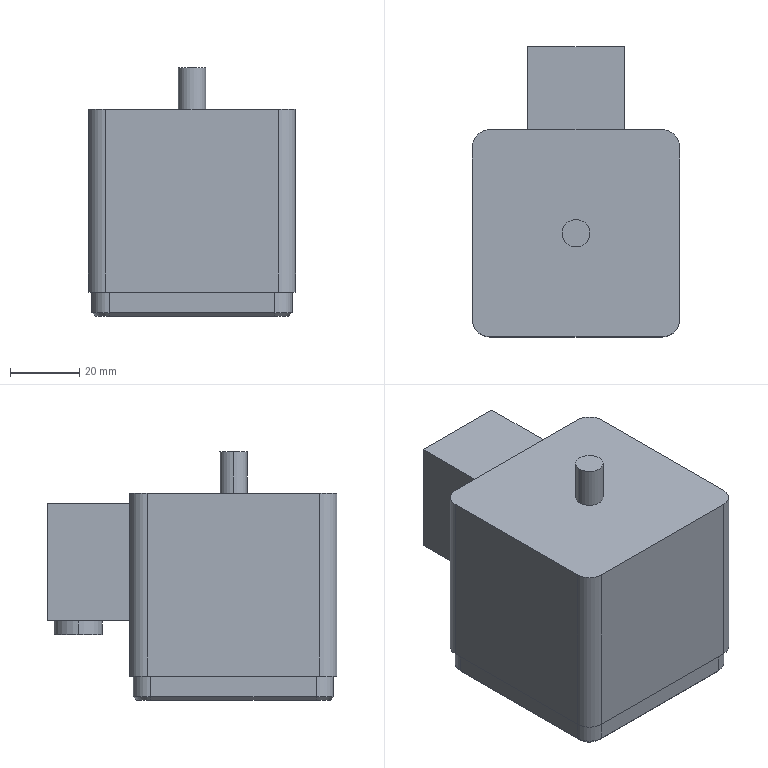Part | SolidWorks | features ICE 4, Fillet 2, Chamfer 1, Extrusion 1 | 1 solid | 38 faces | box 60 x 84 x 72 mm | volume 237017 mm3 | plane 22 | cylinder 12 | cone 4 | commonest cylinder face diameters 10 x8 8 x2 14 x2
STEP:
#1=CARTESIAN_POINT('',(-7.,44.945,23.));
#2=VERTEX_POINT('',#1);
#3=CARTESIAN_POINT('',(7.,44.945,23.));
#4=VERTEX_POINT('',#3);
#5=CARTESIAN_POINT('',(0.,44.945,23.));
#6=DIRECTION('',(0.,0.,-1.));
#7=DIRECTION('',(-1.,0.,0.));
#8=AXIS2_PLACEMENT_3D('',#5,#6,#7);
#9=CIRCLE('',#8,7.);
#10=EDGE_CURVE('',#2,#4,#9,.T.);
#11=ORIENTED_EDGE('',*,*,#10,.T.);
#12=CARTESIAN_POINT('',(7.,44.945,19.));
#13=VERTEX_POINT('',#12);
#14=CARTESIAN_POINT('',(7.,44.945,23.));
#15=DIRECTION('',(0.,0.,-1.));
#16=VECTOR('',#15,1000.);
#17=LINE('',#14,#16);
#18=EDGE_CURVE('',#4,#13,#17,.T.);
#19=ORIENTED_EDGE('',*,*,#18,.T.);
#20=CARTESIAN_POINT('',(-7.,44.945,19.));
#21=VERTEX_POINT('',#20);
#22=CARTESIAN_POINT('',(0.,44.945,19.));
#23=DIRECTION('',(0.,0.,-1.));
#24=DIRECTION('',(-1.,0.,0.));
#25=AXIS2_PLACEMENT_3D('',#22,#23,#24);
#26=CIRCLE('',#25,7.);
#27=EDGE_CURVE('',#21,#13,#26,.T.);
#28=ORIENTED_EDGE('',*,*,#27,.F.);
#29=CARTESIAN_POINT('',(-7.,44.945,23.));
#30=DIRECTION('',(0.,0.,-1.));
#31=VECTOR('',#30,1000.);
#32=LINE('',#29,#31);
#33=EDGE_CURVE('',#2,#21,#32,.T.);
#34=ORIENTED_EDGE('',*,*,#33,.F.);
#35=EDGE_LOOP('',(#11,#19,#28,#34));
#36=FACE_OUTER_BOUND('',#35,.T.);
#37=CARTESIAN_POINT('',(0.,44.945,23.));
#38=DIRECTION('',(0.,0.,-1.));
#39=DIRECTION('',(-1.,0.,0.));
#40=AXIS2_PLACEMENT_3D('',#37,#38,#39);
#41=CYLINDRICAL_SURFACE('',#40,7.);
#42=ADVANCED_FACE('',(#36),#41,.T.);
#43=CARTESIAN_POINT('',(4.,0.,72.));
#44=VERTEX_POINT('',#43);
#45=CARTESIAN_POINT('',(-4.,0.,72.));
#46=VERTEX_POINT('',#45);
#47=CARTESIAN_POINT('',(0.,0.,72.));
#48=DIRECTION('',(0.,0.,1.));
#49=DIRECTION('',(1.,0.,0.));
#50=AXIS2_PLACEMENT_3D('',#47,#48,#49);
#51=CIRCLE('',#50,4.);
#52=EDGE_CURVE('',#44,#46,#51,.T.);
#53=ORIENTED_EDGE('',*,*,#52,.F.);
#54=CARTESIAN_POINT('',(4.,0.,60.));
#55=VERTEX_POINT('',#54);
#56=CARTESIAN_POINT('',(4.,0.,72.));
#57=DIRECTION('',(0.,0.,-1.));
#58=VECTOR('',#57,1000.);
#59=LINE('',#56,#58);
#60=EDGE_CURVE('',#44,#55,#59,.T.);
#61=ORIENTED_EDGE('',*,*,#60,.T.);
#62=CARTESIAN_POINT('',(-4.,0.,60.));
#63=VERTEX_POINT('',#62);
#64=CARTESIAN_POINT('',(0.,0.,60.));
#65=DIRECTION('',(0.,0.,1.));
#66=DIRECTION('',(1.,0.,0.));
#67=AXIS2_PLACEMENT_3D('',#64,#65,#66);
#68=CIRCLE('',#67,4.);
#69=EDGE_CURVE('',#55,#63,#68,.T.);
#70=ORIENTED_EDGE('',*,*,#69,.T.);
#71=CARTESIAN_POINT('',(-4.,0.,72.));
#72=DIRECTION('',(0.,0.,-1.));
#73=VECTOR('',#72,1000.);
#74=LINE('',#71,#73);
#75=EDGE_CURVE('',#46,#63,#74,.T.);
#76=ORIENTED_EDGE('',*,*,#75,.F.);
#77=EDGE_LOOP('',(#53,#61,#70,#76));
#78=FACE_OUTER_BOUND('',#77,.T.);
#79=CARTESIAN_POINT('',(0.,0.,72.));
#80=DIRECTION('',(0.,0.,-1.));
#81=DIRECTION('',(-1.,0.,0.));
#82=AXIS2_PLACEMENT_3D('',#79,#80,#81);
#83=CYLINDRICAL_SURFACE('',#82,4.);
#84=ADVANCED_FACE('',(#78),#83,.T.);
#85=CARTESIAN_POINT('',(14.,54.,23.));
#86=VERTEX_POINT('',#85);
#87=CARTESIAN_POINT('',(14.,30.,23.));
#88=VERTEX_POINT('',#87);
#89=CARTESIAN_POINT('',(14.,54.,23.));
#90=DIRECTION('',(0.,-1.,0.));
#91=VECTOR('',#90,1000.);
#92=LINE('',#89,#91);
#93=EDGE_CURVE('',#86,#88,#92,.T.);
#94=ORIENTED_EDGE('',*,*,#93,.F.);
#95=CARTESIAN_POINT('',(14.,54.,57.));
#96=VERTEX_POINT('',#95);
#97=CARTESIAN_POINT('',(14.,54.,57.));
#98=DIRECTION('',(0.,0.,-1.));
#99=VECTOR('',#98,1000.);
#100=LINE('',#97,#99);
#101=EDGE_CURVE('',#96,#86,#100,.T.);
#102=ORIENTED_EDGE('',*,*,#101,.F.);
#103=CARTESIAN_POINT('',(14.,30.,57.));
#104=VERTEX_POINT('',#103);
#105=CARTESIAN_POINT('',(14.,54.,57.));
#106=DIRECTION('',(0.,-1.,0.));
#107=VECTOR('',#106,1000.);
#108=LINE('',#105,#107);
#109=EDGE_CURVE('',#96,#104,#108,.T.);
#110=ORIENTED_EDGE('',*,*,#109,.T.);
#111=CARTESIAN_POINT('',(14.,30.,57.));
#112=DIRECTION('',(0.,0.,-1.));
#113=VECTOR('',#112,1000.);
#114=LINE('',#111,#113);
#115=EDGE_CURVE('',#104,#88,#114,.T.);
#116=ORIENTED_EDGE('',*,*,#115,.T.);
#117=EDGE_LOOP('',(#94,#102,#110,#116));
#118=FACE_OUTER_BOUND('',#117,.T.);
#119=CARTESIAN_POINT('',(14.,54.,57.));
#120=DIRECTION('',(-1.,0.,0.));
#121=DIRECTION('',(0.,0.,1.));
#122=AXIS2_PLACEMENT_3D('',#119,#120,#121);
#123=PLANE('',#122);
#124=ADVANCED_FACE('',(#118),#123,.F.);
#125=CARTESIAN_POINT('',(-14.,30.,23.));
#126=VERTEX_POINT('',#125);
#127=CARTESIAN_POINT('',(-14.,54.,23.));
#128=VERTEX_POINT('',#127);
#129=CARTESIAN_POINT('',(-14.,54.,23.));
#130=DIRECTION('',(0.,1.,0.));
#131=VECTOR('',#130,1000.);
#132=LINE('',#129,#131);
#133=EDGE_CURVE('',#126,#128,#132,.T.);
#134=ORIENTED_EDGE('',*,*,#133,.F.);
#135=CARTESIAN_POINT('',(-14.,30.,57.));
#136=VERTEX_POINT('',#135);
#137=CARTESIAN_POINT('',(-14.,30.,57.));
#138=DIRECTION('',(0.,0.,1.));
#139=VECTOR('',#138,1000.);
#140=LINE('',#137,#139);
#141=EDGE_CURVE('',#126,#136,#140,.T.);
#142=ORIENTED_EDGE('',*,*,#141,.T.);
#143=CARTESIAN_POINT('',(-14.,54.,57.));
#144=VERTEX_POINT('',#143);
#145=CARTESIAN_POINT('',(-14.,54.,57.));
#146=DIRECTION('',(0.,-1.,0.));
#147=VECTOR('',#146,1000.);
#148=LINE('',#145,#147);
#149=EDGE_CURVE('',#144,#136,#148,.T.);
#150=ORIENTED_EDGE('',*,*,#149,.F.);
#151=CARTESIAN_POINT('',(-14.,54.,57.));
#152=DIRECTION('',(0.,0.,1.));
#153=VECTOR('',#152,1000.);
#154=LINE('',#151,#153);
#155=EDGE_CURVE('',#128,#144,#154,.T.);
#156=ORIENTED_EDGE('',*,*,#155,.F.);
#157=EDGE_LOOP('',(#134,#142,#150,#156));
#158=FACE_OUTER_BOUND('',#157,.T.);
#159=CARTESIAN_POINT('',(-14.,54.,57.));
#160=DIRECTION('',(1.,0.,0.));
#161=DIRECTION('',(0.,0.,-1.));
#162=AXIS2_PLACEMENT_3D('',#159,#160,#161);
#163=PLANE('',#162);
#164=ADVANCED_FACE('',(#158),#163,.F.);
#165=CARTESIAN_POINT('',(0.,54.,23.));
#166=DIRECTION('',(1.,0.,0.));
#167=VECTOR('',#166,1000.);
#168=LINE('',#165,#167);
#169=EDGE_CURVE('',#128,#86,#168,.T.);
#170=ORIENTED_EDGE('',*,*,#169,.F.);
#171=ORIENTED_EDGE('',*,*,#155,.T.);
#172=CARTESIAN_POINT('',(14.,54.,57.));
#173=DIRECTION('',(1.,0.,0.));
#174=VECTOR('',#173,1000.);
#175=LINE('',#172,#174);
#176=EDGE_CURVE('',#144,#96,#175,.T.);
#177=ORIENTED_EDGE('',*,*,#176,.T.);
#178=ORIENTED_EDGE('',*,*,#101,.T.);
#179=EDGE_LOOP('',(#170,#171,#177,#178));
#180=FACE_OUTER_BOUND('',#179,.T.);
#181=CARTESIAN_POINT('',(0.,54.,0.));
#182=DIRECTION('',(0.,-1.,0.));
#183=DIRECTION('',(0.,0.,-1.));
#184=AXIS2_PLACEMENT_3D('',#181,#182,#183);
#185=PLANE('',#184);
#186=ADVANCED_FACE('',(#180),#185,.F.);
#187=ORIENTED_EDGE('',*,*,#141,.F.);
#188=CARTESIAN_POINT('',(22.114,30.,23.));
#189=DIRECTION('',(-1.,0.,0.));
#190=VECTOR('',#189,1000.);
#191=LINE('',#188,#190);
#192=EDGE_CURVE('',#88,#126,#191,.T.);
#193=ORIENTED_EDGE('',*,*,#192,.F.);
#194=ORIENTED_EDGE('',*,*,#115,.F.);
#195=CARTESIAN_POINT('',(14.,30.,57.));
#196=DIRECTION('',(1.,0.,0.));
#197=VECTOR('',#196,1000.);
#198=LINE('',#195,#197);
#199=EDGE_CURVE('',#136,#104,#198,.T.);
#200=ORIENTED_EDGE('',*,*,#199,.F.);
#201=EDGE_LOOP('',(#187,#193,#194,#200));
#202=FACE_BOUND('',#201,.T.);
#203=CARTESIAN_POINT('',(-25.,30.,7.));
#204=VERTEX_POINT('',#203);
#205=CARTESIAN_POINT('',(25.,30.,7.));
#206=VERTEX_POINT('',#205);
#207=CARTESIAN_POINT('',(30.,30.,7.));
#208=DIRECTION('',(1.,0.,0.));
#209=VECTOR('',#208,1000.);
#210=LINE('',#207,#209);
#211=EDGE_CURVE('',#204,#206,#210,.T.);
#212=ORIENTED_EDGE('',*,*,#211,.F.);
#213=CARTESIAN_POINT('',(-25.,30.,60.));
#214=VERTEX_POINT('',#213);
#215=CARTESIAN_POINT('',(-25.,30.,60.));
#216=DIRECTION('',(0.,0.,1.));
#217=VECTOR('',#216,1000.);
#218=LINE('',#215,#217);
#219=EDGE_CURVE('',#204,#214,#218,.T.);
#220=ORIENTED_EDGE('',*,*,#219,.T.);
#221=CARTESIAN_POINT('',(25.,30.,60.));
#222=VERTEX_POINT('',#221);
#223=CARTESIAN_POINT('',(-30.,30.,60.));
#224=DIRECTION('',(-1.,0.,0.));
#225=VECTOR('',#224,1000.);
#226=LINE('',#223,#225);
#227=EDGE_CURVE('',#222,#214,#226,.T.);
#228=ORIENTED_EDGE('',*,*,#227,.F.);
#229=CARTESIAN_POINT('',(25.,30.,60.));
#230=DIRECTION('',(0.,0.,-1.));
#231=VECTOR('',#230,1000.);
#232=LINE('',#229,#231);
#233=EDGE_CURVE('',#222,#206,#232,.T.);
#234=ORIENTED_EDGE('',*,*,#233,.T.);
#235=EDGE_LOOP('',(#212,#220,#228,#234));
#236=FACE_OUTER_BOUND('',#235,.T.);
#237=CARTESIAN_POINT('',(-30.,30.,60.));
#238=DIRECTION('',(0.,-1.,0.));
#239=DIRECTION('',(0.,0.,-1.));
#240=AXIS2_PLACEMENT_3D('',#237,#238,#239);
#241=PLANE('',#240);
#242=ADVANCED_FACE('',(#202,#236),#241,.F.);
#243=CARTESIAN_POINT('',(30.,-25.,60.));
#244=VERTEX_POINT('',#243);
#245=CARTESIAN_POINT('',(30.,25.,60.));
#246=VERTEX_POINT('',#245);
#247=CARTESIAN_POINT('',(30.,30.,60.));
#248=DIRECTION('',(0.,1.,0.));
#249=VECTOR('',#248,1000.);
#250=LINE('',#247,#249);
#251=EDGE_CURVE('',#244,#246,#250,.T.);
#252=ORIENTED_EDGE('',*,*,#251,.F.);
#253=CARTESIAN_POINT('',(30.,-25.,7.));
#254=VERTEX_POINT('',#253);
#255=CARTESIAN_POINT('',(30.,-25.,60.));
#256=DIRECTION('',(0.,0.,-1.));
#257=VECTOR('',#256,1000.);
#258=LINE('',#255,#257);
#259=EDGE_CURVE('',#244,#254,#258,.T.);
#260=ORIENTED_EDGE('',*,*,#259,.T.);
#261=CARTESIAN_POINT('',(30.,25.,7.));
#262=VERTEX_POINT('',#261);
#263=CARTESIAN_POINT('',(30.,30.,7.));
#264=DIRECTION('',(0.,-1.,0.));
#265=VECTOR('',#264,1000.);
#266=LINE('',#263,#265);
#267=EDGE_CURVE('',#262,#254,#266,.T.);
#268=ORIENTED_EDGE('',*,*,#267,.F.);
#269=CARTESIAN_POINT('',(30.,25.,60.));
#270=DIRECTION('',(0.,0.,1.));
#271=VECTOR('',#270,1000.);
#272=LINE('',#269,#271);
#273=EDGE_CURVE('',#262,#246,#272,.T.);
#274=ORIENTED_EDGE('',*,*,#273,.T.);
#275=EDGE_LOOP('',(#252,#260,#268,#274));
#276=FACE_OUTER_BOUND('',#275,.T.);
#277=CARTESIAN_POINT('',(30.,30.,60.));
#278=DIRECTION('',(-1.,0.,0.));
#279=DIRECTION('',(0.,-1.,0.));
#280=AXIS2_PLACEMENT_3D('',#277,#278,#279);
#281=PLANE('',#280);
#282=ADVANCED_FACE('',(#276),#281,.F.);
#283=CARTESIAN_POINT('',(-30.,-25.,7.));
#284=VERTEX_POINT('',#283);
#285=CARTESIAN_POINT('',(-30.,25.,7.));
#286=VERTEX_POINT('',#285);
#287=CARTESIAN_POINT('',(-30.,30.,7.));
#288=DIRECTION('',(0.,1.,0.));
#289=VECTOR('',#288,1000.);
#290=LINE('',#287,#289);
#291=EDGE_CURVE('',#284,#286,#290,.T.);
#292=ORIENTED_EDGE('',*,*,#291,.F.);
#293=CARTESIAN_POINT('',(-30.,-25.,60.));
#294=VERTEX_POINT('',#293);
#295=CARTESIAN_POINT('',(-30.,-25.,60.));
#296=DIRECTION('',(0.,0.,1.));
#297=VECTOR('',#296,1000.);
#298=LINE('',#295,#297);
#299=EDGE_CURVE('',#284,#294,#298,.T.);
#300=ORIENTED_EDGE('',*,*,#299,.T.);
#301=CARTESIAN_POINT('',(-30.,25.,60.));
#302=VERTEX_POINT('',#301);
#303=CARTESIAN_POINT('',(-30.,30.,60.));
#304=DIRECTION('',(0.,-1.,0.));
#305=VECTOR('',#304,1000.);
#306=LINE('',#303,#305);
#307=EDGE_CURVE('',#302,#294,#306,.T.);
#308=ORIENTED_EDGE('',*,*,#307,.F.);
#309=CARTESIAN_POINT('',(-30.,25.,60.));
#310=DIRECTION('',(0.,0.,-1.));
#311=VECTOR('',#310,1000.);
#312=LINE('',#309,#311);
#313=EDGE_CURVE('',#302,#286,#312,.T.);
#314=ORIENTED_EDGE('',*,*,#313,.T.);
#315=EDGE_LOOP('',(#292,#300,#308,#314));
#316=FACE_OUTER_BOUND('',#315,.T.);
#317=CARTESIAN_POINT('',(-30.,30.,60.));
#318=DIRECTION('',(1.,0.,0.));
#319=DIRECTION('',(0.,1.,0.));
#320=AXIS2_PLACEMENT_3D('',#317,#318,#319);
#321=PLANE('',#320);
#322=ADVANCED_FACE('',(#316),#321,.F.);
#323=CARTESIAN_POINT('',(25.,-30.,7.));
#324=VERTEX_POINT('',#323);
#325=CARTESIAN_POINT('',(-25.,-30.,7.));
#326=VERTEX_POINT('',#325);
#327=CARTESIAN_POINT('',(30.,-30.,7.));
#328=DIRECTION('',(-1.,0.,0.));
#329=VECTOR('',#328,1000.);
#330=LINE('',#327,#329);
#331=EDGE_CURVE('',#324,#326,#330,.T.);
#332=ORIENTED_EDGE('',*,*,#331,.F.);
#333=CARTESIAN_POINT('',(25.,-30.,60.));
#334=VERTEX_POINT('',#333);
#335=CARTESIAN_POINT('',(25.,-30.,60.));
#336=DIRECTION('',(0.,0.,1.));
#337=VECTOR('',#336,1000.);
#338=LINE('',#335,#337);
#339=EDGE_CURVE('',#324,#334,#338,.T.);
#340=ORIENTED_EDGE('',*,*,#339,.T.);
#341=CARTESIAN_POINT('',(-25.,-30.,60.));
#342=VERTEX_POINT('',#341);
#343=CARTESIAN_POINT('',(-30.,-30.,60.));
#344=DIRECTION('',(1.,0.,0.));
#345=VECTOR('',#344,1000.);
#346=LINE('',#343,#345);
#347=EDGE_CURVE('',#342,#334,#346,.T.);
#348=ORIENTED_EDGE('',*,*,#347,.F.);
#349=CARTESIAN_POINT('',(-25.,-30.,60.));
#350=DIRECTION('',(0.,0.,-1.));
#351=VECTOR('',#350,1000.);
#352=LINE('',#349,#351);
#353=EDGE_CURVE('',#342,#326,#352,.T.);
#354=ORIENTED_EDGE('',*,*,#353,.T.);
#355=EDGE_LOOP('',(#332,#340,#348,#354));
#356=FACE_OUTER_BOUND('',#355,.T.);
#357=CARTESIAN_POINT('',(-30.,-30.,60.));
#358=DIRECTION('',(0.,1.,0.));
#359=DIRECTION('',(0.,0.,1.));
#360=AXIS2_PLACEMENT_3D('',#357,#358,#359);
#361=PLANE('',#360);
#362=ADVANCED_FACE('',(#356),#361,.F.);
#363=CARTESIAN_POINT('',(0.,0.,60.));
#364=DIRECTION('',(0.,0.,1.));
#365=DIRECTION('',(1.,0.,0.));
#366=AXIS2_PLACEMENT_3D('',#363,#364,#365);
#367=CIRCLE('',#366,4.);
#368=EDGE_CURVE('',#63,#55,#367,.T.);
#369=ORIENTED_EDGE('',*,*,#368,.F.);
#370=ORIENTED_EDGE('',*,*,#69,.F.);
#371=EDGE_LOOP('',(#369,#370));
#372=FACE_BOUND('',#371,.T.);
#373=ORIENTED_EDGE('',*,*,#347,.T.);
#374=CARTESIAN_POINT('',(25.,-25.,60.));
#375=DIRECTION('',(0.,0.,1.));
#376=DIRECTION('',(1.,0.,0.));
#377=AXIS2_PLACEMENT_3D('',#374,#375,#376);
#378=CIRCLE('',#377,5.);
#379=EDGE_CURVE('',#334,#244,#378,.T.);
#380=ORIENTED_EDGE('',*,*,#379,.T.);
#381=ORIENTED_EDGE('',*,*,#251,.T.);
#382=CARTESIAN_POINT('',(25.,25.,60.));
#383=DIRECTION('',(0.,0.,1.));
#384=DIRECTION('',(1.,0.,0.));
#385=AXIS2_PLACEMENT_3D('',#382,#383,#384);
#386=CIRCLE('',#385,5.);
#387=EDGE_CURVE('',#246,#222,#386,.T.);
#388=ORIENTED_EDGE('',*,*,#387,.T.);
#389=ORIENTED_EDGE('',*,*,#227,.T.);
#390=CARTESIAN_POINT('',(-25.,25.,60.));
#391=DIRECTION('',(0.,0.,1.));
#392=DIRECTION('',(1.,0.,0.));
#393=AXIS2_PLACEMENT_3D('',#390,#391,#392);
#394=CIRCLE('',#393,5.);
#395=EDGE_CURVE('',#214,#302,#394,.T.);
#396=ORIENTED_EDGE('',*,*,#395,.T.);
#397=ORIENTED_EDGE('',*,*,#307,.T.);
#398=CARTESIAN_POINT('',(-25.,-25.,60.));
#399=DIRECTION('',(0.,0.,1.));
#400=DIRECTION('',(1.,0.,0.));
#401=AXIS2_PLACEMENT_3D('',#398,#399,#400);
#402=CIRCLE('',#401,5.);
#403=EDGE_CURVE('',#294,#342,#402,.T.);
#404=ORIENTED_EDGE('',*,*,#403,.T.);
#405=EDGE_LOOP('',(#373,#380,#381,#388,#389,#396,#397,#404));
#406=FACE_OUTER_BOUND('',#405,.T.);
#407=CARTESIAN_POINT('',(0.,0.,60.));
#408=DIRECTION('',(0.,0.,1.));
#409=DIRECTION('',(1.,0.,0.));
#410=AXIS2_PLACEMENT_3D('',#407,#408,#409);
#411=PLANE('',#410);
#412=ADVANCED_FACE('',(#372,#406),#411,.T.);
#413=ORIENTED_EDGE('',*,*,#60,.F.);
#414=CARTESIAN_POINT('',(0.,0.,72.));
#415=DIRECTION('',(0.,0.,1.));
#416=DIRECTION('',(1.,0.,0.));
#417=AXIS2_PLACEMENT_3D('',#414,#415,#416);
#418=CIRCLE('',#417,4.);
#419=EDGE_CURVE('',#46,#44,#418,.T.);
#420=ORIENTED_EDGE('',*,*,#419,.F.);
#421=ORIENTED_EDGE('',*,*,#75,.T.);
#422=ORIENTED_EDGE('',*,*,#368,.T.);
#423=EDGE_LOOP('',(#413,#420,#421,#422));
#424=FACE_OUTER_BOUND('',#423,.T.);
#425=CARTESIAN_POINT('',(0.,0.,72.));
#426=DIRECTION('',(0.,0.,-1.));
#427=DIRECTION('',(-1.,0.,0.));
#428=AXIS2_PLACEMENT_3D('',#425,#426,#427);
#429=CYLINDRICAL_SURFACE('',#428,4.);
#430=ADVANCED_FACE('',(#424),#429,.T.);
#431=ORIENTED_EDGE('',*,*,#419,.T.);
#432=ORIENTED_EDGE('',*,*,#52,.T.);
#433=EDGE_LOOP('',(#431,#432));
#434=FACE_OUTER_BOUND('',#433,.T.);
#435=CARTESIAN_POINT('',(0.,0.,72.));
#436=DIRECTION('',(0.,0.,1.));
#437=DIRECTION('',(1.,0.,0.));
#438=AXIS2_PLACEMENT_3D('',#435,#436,#437);
#439=PLANE('',#438);
#440=ADVANCED_FACE('',(#434),#439,.T.);
#441=CARTESIAN_POINT('',(24.,-29.,7.));
#442=VERTEX_POINT('',#441);
#443=CARTESIAN_POINT('',(-24.,-29.,7.));
#444=VERTEX_POINT('',#443);
#445=CARTESIAN_POINT('',(29.,-29.,7.));
#446=DIRECTION('',(-1.,0.,0.));
#447=VECTOR('',#446,1000.);
#448=LINE('',#445,#447);
#449=EDGE_CURVE('',#442,#444,#448,.T.);
#450=ORIENTED_EDGE('',*,*,#449,.F.);
#451=CARTESIAN_POINT('',(29.,-24.,7.));
#452=VERTEX_POINT('',#451);
#453=CARTESIAN_POINT('',(24.,-24.,7.));
#454=DIRECTION('',(0.,0.,1.));
#455=DIRECTION('',(-1.,0.,0.));
#456=AXIS2_PLACEMENT_3D('',#453,#454,#455);
#457=CIRCLE('',#456,5.);
#458=EDGE_CURVE('',#442,#452,#457,.T.);
#459=ORIENTED_EDGE('',*,*,#458,.T.);
#460=CARTESIAN_POINT('',(29.,24.,7.));
#461=VERTEX_POINT('',#460);
#462=CARTESIAN_POINT('',(29.,29.,7.));
#463=DIRECTION('',(0.,-1.,0.));
#464=VECTOR('',#463,1000.);
#465=LINE('',#462,#464);
#466=EDGE_CURVE('',#461,#452,#465,.T.);
#467=ORIENTED_EDGE('',*,*,#466,.F.);
#468=CARTESIAN_POINT('',(24.,29.,7.));
#469=VERTEX_POINT('',#468);
#470=CARTESIAN_POINT('',(24.,24.,7.));
#471=DIRECTION('',(0.,0.,1.));
#472=DIRECTION('',(-1.,0.,0.));
#473=AXIS2_PLACEMENT_3D('',#470,#471,#472);
#474=CIRCLE('',#473,5.);
#475=EDGE_CURVE('',#461,#469,#474,.T.);
#476=ORIENTED_EDGE('',*,*,#475,.T.);
#477=CARTESIAN_POINT('',(-24.,29.,7.));
#478=VERTEX_POINT('',#477);
#479=CARTESIAN_POINT('',(29.,29.,7.));
#480=DIRECTION('',(1.,0.,0.));
#481=VECTOR('',#480,1000.);
#482=LINE('',#479,#481);
#483=EDGE_CURVE('',#478,#469,#482,.T.);
#484=ORIENTED_EDGE('',*,*,#483,.F.);
#485=CARTESIAN_POINT('',(-29.,24.,7.));
#486=VERTEX_POINT('',#485);
#487=CARTESIAN_POINT('',(-24.,24.,7.));
#488=DIRECTION('',(0.,0.,1.));
#489=DIRECTION('',(-1.,0.,0.));
#490=AXIS2_PLACEMENT_3D('',#487,#488,#489);
#491=CIRCLE('',#490,5.);
#492=EDGE_CURVE('',#478,#486,#491,.T.);
#493=ORIENTED_EDGE('',*,*,#492,.T.);
#494=CARTESIAN_POINT('',(-29.,-24.,7.));
#495=VERTEX_POINT('',#494);
#496=CARTESIAN_POINT('',(-29.,29.,7.));
#497=DIRECTION('',(0.,1.,0.));
#498=VECTOR('',#497,1000.);
#499=LINE('',#496,#498);
#500=EDGE_CURVE('',#495,#486,#499,.T.);
#501=ORIENTED_EDGE('',*,*,#500,.F.);
#502=CARTESIAN_POINT('',(-24.,-24.,7.));
#503=DIRECTION('',(0.,0.,1.));
#504=DIRECTION('',(-1.,0.,0.));
#505=AXIS2_PLACEMENT_3D('',#502,#503,#504);
#506=CIRCLE('',#505,5.);
#507=EDGE_CURVE('',#495,#444,#506,.T.);
#508=ORIENTED_EDGE('',*,*,#507,.T.);
#509=EDGE_LOOP('',(#450,#459,#467,#476,#484,#493,#501,#508));
#510=FACE_BOUND('',#509,.T.);
#511=ORIENTED_EDGE('',*,*,#267,.T.);
#512=CARTESIAN_POINT('',(25.,-25.,7.));
#513=DIRECTION('',(0.,0.,-1.));
#514=DIRECTION('',(-1.,0.,0.));
#515=AXIS2_PLACEMENT_3D('',#512,#513,#514);
#516=CIRCLE('',#515,5.);
#517=EDGE_CURVE('',#254,#324,#516,.T.);
#518=ORIENTED_EDGE('',*,*,#517,.T.);
#519=ORIENTED_EDGE('',*,*,#331,.T.);
#520=CARTESIAN_POINT('',(-25.,-25.,7.));
#521=DIRECTION('',(0.,0.,-1.));
#522=DIRECTION('',(-1.,0.,0.));
#523=AXIS2_PLACEMENT_3D('',#520,#521,#522);
#524=CIRCLE('',#523,5.);
#525=EDGE_CURVE('',#326,#284,#524,.T.);
#526=ORIENTED_EDGE('',*,*,#525,.T.);
#527=ORIENTED_EDGE('',*,*,#291,.T.);
#528=CARTESIAN_POINT('',(-25.,25.,7.));
#529=DIRECTION('',(0.,0.,-1.));
#530=DIRECTION('',(-1.,0.,0.));
#531=AXIS2_PLACEMENT_3D('',#528,#529,#530);
#532=CIRCLE('',#531,5.);
#533=EDGE_CURVE('',#286,#204,#532,.T.);
#534=ORIENTED_EDGE('',*,*,#533,.T.);
#535=ORIENTED_EDGE('',*,*,#211,.T.);
#536=CARTESIAN_POINT('',(25.,25.,7.));
#537=DIRECTION('',(0.,0.,-1.));
#538=DIRECTION('',(-1.,0.,0.));
#539=AXIS2_PLACEMENT_3D('',#536,#537,#538);
#540=CIRCLE('',#539,5.);
#541=EDGE_CURVE('',#206,#262,#540,.T.);
#542=ORIENTED_EDGE('',*,*,#541,.T.);
#543=EDGE_LOOP('',(#511,#518,#519,#526,#527,#534,#535,#542));
#544=FACE_OUTER_BOUND('',#543,.T.);
#545=CARTESIAN_POINT('',(0.,0.,7.));
#546=DIRECTION('',(0.,0.,-1.));
#547=DIRECTION('',(-1.,0.,0.));
#548=AXIS2_PLACEMENT_3D('',#545,#546,#547);
#549=PLANE('',#548);
#550=ADVANCED_FACE('',(#510,#544),#549,.T.);
#551=CARTESIAN_POINT('',(-29.,24.,1.));
#552=VERTEX_POINT('',#551);
#553=CARTESIAN_POINT('',(-29.,24.,7.));
#554=DIRECTION('',(0.,0.,-1.));
#555=VECTOR('',#554,1000.);
#556=LINE('',#553,#555);
#557=EDGE_CURVE('',#486,#552,#556,.T.);
#558=ORIENTED_EDGE('',*,*,#557,.T.);
#559=CARTESIAN_POINT('',(-29.,-24.,1.));
#560=VERTEX_POINT('',#559);
#561=CARTESIAN_POINT('',(-29.,-24.,1.));
#562=DIRECTION('',(0.,-1.,0.));
#563=VECTOR('',#562,1000.);
#564=LINE('',#561,#563);
#565=EDGE_CURVE('',#552,#560,#564,.T.);
#566=ORIENTED_EDGE('',*,*,#565,.T.);
#567=CARTESIAN_POINT('',(-29.,-24.,7.));
#568=DIRECTION('',(0.,0.,1.));
#569=VECTOR('',#568,1000.);
#570=LINE('',#567,#569);
#571=EDGE_CURVE('',#560,#495,#570,.T.);
#572=ORIENTED_EDGE('',*,*,#571,.T.);
#573=ORIENTED_EDGE('',*,*,#500,.T.);
#574=EDGE_LOOP('',(#558,#566,#572,#573));
#575=FACE_OUTER_BOUND('',#574,.T.);
#576=CARTESIAN_POINT('',(-29.,29.,7.));
#577=DIRECTION('',(-1.,0.,0.));
#578=DIRECTION('',(0.,-1.,0.));
#579=AXIS2_PLACEMENT_3D('',#576,#577,#578);
#580=PLANE('',#579);
#581=ADVANCED_FACE('',(#575),#580,.T.);
#582=CARTESIAN_POINT('',(-24.,-29.,1.));
#583=VERTEX_POINT('',#582);
#584=CARTESIAN_POINT('',(-24.,-29.,7.));
#585=DIRECTION('',(0.,0.,-1.));
#586=VECTOR('',#585,1000.);
#587=LINE('',#584,#586);
#588=EDGE_CURVE('',#444,#583,#587,.T.);
#589=ORIENTED_EDGE('',*,*,#588,.T.);
#590=CARTESIAN_POINT('',(24.,-29.,1.));
#591=VERTEX_POINT('',#590);
#592=CARTESIAN_POINT('',(24.,-29.,1.));
#593=DIRECTION('',(1.,0.,0.));
#594=VECTOR('',#593,1000.);
#595=LINE('',#592,#594);
#596=EDGE_CURVE('',#583,#591,#595,.T.);
#597=ORIENTED_EDGE('',*,*,#596,.T.);
#598=CARTESIAN_POINT('',(24.,-29.,7.));
#599=DIRECTION('',(0.,0.,1.));
#600=VECTOR('',#599,1000.);
#601=LINE('',#598,#600);
#602=EDGE_CURVE('',#591,#442,#601,.T.);
#603=ORIENTED_EDGE('',*,*,#602,.T.);
#604=ORIENTED_EDGE('',*,*,#449,.T.);
#605=EDGE_LOOP('',(#589,#597,#603,#604));
#606=FACE_OUTER_BOUND('',#605,.T.);
#607=CARTESIAN_POINT('',(29.,-29.,7.));
#608=DIRECTION('',(0.,-1.,0.));
#609=DIRECTION('',(0.,0.,-1.));
#610=AXIS2_PLACEMENT_3D('',#607,#608,#609);
#611=PLANE('',#610);
#612=ADVANCED_FACE('',(#606),#611,.T.);
#613=CARTESIAN_POINT('',(29.,-24.,1.));
#614=VERTEX_POINT('',#613);
#615=CARTESIAN_POINT('',(29.,-24.,7.));
#616=DIRECTION('',(0.,0.,-1.));
#617=VECTOR('',#616,1000.);
#618=LINE('',#615,#617);
#619=EDGE_CURVE('',#452,#614,#618,.T.);
#620=ORIENTED_EDGE('',*,*,#619,.T.);
#621=CARTESIAN_POINT('',(29.,24.,1.));
#622=VERTEX_POINT('',#621);
#623=CARTESIAN_POINT('',(29.,24.,1.));
#624=DIRECTION('',(0.,1.,0.));
#625=VECTOR('',#624,1000.);
#626=LINE('',#623,#625);
#627=EDGE_CURVE('',#614,#622,#626,.T.);
#628=ORIENTED_EDGE('',*,*,#627,.T.);
#629=CARTESIAN_POINT('',(29.,24.,7.));
#630=DIRECTION('',(0.,0.,1.));
#631=VECTOR('',#630,1000.);
#632=LINE('',#629,#631);
#633=EDGE_CURVE('',#622,#461,#632,.T.);
#634=ORIENTED_EDGE('',*,*,#633,.T.);
#635=ORIENTED_EDGE('',*,*,#466,.T.);
#636=EDGE_LOOP('',(#620,#628,#634,#635));
#637=FACE_OUTER_BOUND('',#636,.T.);
#638=CARTESIAN_POINT('',(29.,29.,7.));
#639=DIRECTION('',(1.,0.,0.));
#640=DIRECTION('',(0.,1.,0.));
#641=AXIS2_PLACEMENT_3D('',#638,#639,#640);
#642=PLANE('',#641);
#643=ADVANCED_FACE('',(#637),#642,.T.);
#644=CARTESIAN_POINT('',(24.,29.,1.));
#645=VERTEX_POINT('',#644);
#646=CARTESIAN_POINT('',(24.,29.,7.));
#647=DIRECTION('',(0.,0.,-1.));
#648=VECTOR('',#647,1000.);
#649=LINE('',#646,#648);
#650=EDGE_CURVE('',#469,#645,#649,.T.);
#651=ORIENTED_EDGE('',*,*,#650,.T.);
#652=CARTESIAN_POINT('',(-24.,29.,1.));
#653=VERTEX_POINT('',#652);
#654=CARTESIAN_POINT('',(-24.,29.,1.));
#655=DIRECTION('',(-1.,0.,0.));
#656=VECTOR('',#655,1000.);
#657=LINE('',#654,#656);
#658=EDGE_CURVE('',#645,#653,#657,.T.);
#659=ORIENTED_EDGE('',*,*,#658,.T.);
#660=CARTESIAN_POINT('',(-24.,29.,7.));
#661=DIRECTION('',(0.,0.,1.));
#662=VECTOR('',#661,1000.);
#663=LINE('',#660,#662);
#664=EDGE_CURVE('',#653,#478,#663,.T.);
#665=ORIENTED_EDGE('',*,*,#664,.T.);
#666=ORIENTED_EDGE('',*,*,#483,.T.);
#667=EDGE_LOOP('',(#651,#659,#665,#666));
#668=FACE_OUTER_BOUND('',#667,.T.);
#669=CARTESIAN_POINT('',(29.,29.,7.));
#670=DIRECTION('',(0.,1.,0.));
#671=DIRECTION('',(0.,0.,1.));
#672=AXIS2_PLACEMENT_3D('',#669,#670,#671);
#673=PLANE('',#672);
#674=ADVANCED_FACE('',(#668),#673,.T.);
#675=CARTESIAN_POINT('',(24.,-28.,0.));
#676=VERTEX_POINT('',#675);
#677=CARTESIAN_POINT('',(-24.,-28.,0.));
#678=VERTEX_POINT('',#677);
#679=CARTESIAN_POINT('',(-24.,-28.,0.));
#680=DIRECTION('',(-1.,0.,0.));
#681=VECTOR('',#680,1000.);
#682=LINE('',#679,#681);
#683=EDGE_CURVE('',#676,#678,#682,.T.);
#684=ORIENTED_EDGE('',*,*,#683,.T.);
#685=CARTESIAN_POINT('',(-28.,-24.,0.));
#686=VERTEX_POINT('',#685);
#687=CARTESIAN_POINT('',(-24.,-24.,0.));
#688=DIRECTION('',(0.,0.,-1.));
#689=DIRECTION('',(1.,0.,0.));
#690=AXIS2_PLACEMENT_3D('',#687,#688,#689);
#691=CIRCLE('',#690,4.);
#692=EDGE_CURVE('',#678,#686,#691,.T.);
#693=ORIENTED_EDGE('',*,*,#692,.T.);
#694=CARTESIAN_POINT('',(-28.,24.,0.));
#695=VERTEX_POINT('',#694);
#696=CARTESIAN_POINT('',(-28.,24.,0.));
#697=DIRECTION('',(0.,1.,0.));
#698=VECTOR('',#697,1000.);
#699=LINE('',#696,#698);
#700=EDGE_CURVE('',#686,#695,#699,.T.);
#701=ORIENTED_EDGE('',*,*,#700,.T.);
#702=CARTESIAN_POINT('',(-24.,28.,0.));
#703=VERTEX_POINT('',#702);
#704=CARTESIAN_POINT('',(-24.,24.,0.));
#705=DIRECTION('',(0.,0.,-1.));
#706=DIRECTION('',(1.,0.,0.));
#707=AXIS2_PLACEMENT_3D('',#704,#705,#706);
#708=CIRCLE('',#707,4.);
#709=EDGE_CURVE('',#695,#703,#708,.T.);
#710=ORIENTED_EDGE('',*,*,#709,.T.);
#711=CARTESIAN_POINT('',(24.,28.,0.));
#712=VERTEX_POINT('',#711);
#713=CARTESIAN_POINT('',(24.,28.,0.));
#714=DIRECTION('',(1.,0.,0.));
#715=VECTOR('',#714,1000.);
#716=LINE('',#713,#715);
#717=EDGE_CURVE('',#703,#712,#716,.T.);
#718=ORIENTED_EDGE('',*,*,#717,.T.);
#719=CARTESIAN_POINT('',(28.,24.,0.));
#720=VERTEX_POINT('',#719);
#721=CARTESIAN_POINT('',(24.,24.,0.));
#722=DIRECTION('',(0.,0.,-1.));
#723=DIRECTION('',(1.,0.,0.));
#724=AXIS2_PLACEMENT_3D('',#721,#722,#723);
#725=CIRCLE('',#724,4.);
#726=EDGE_CURVE('',#712,#720,#725,.T.);
#727=ORIENTED_EDGE('',*,*,#726,.T.);
#728=CARTESIAN_POINT('',(28.,-24.,0.));
#729=VERTEX_POINT('',#728);
#730=CARTESIAN_POINT('',(28.,-24.,0.));
#731=DIRECTION('',(0.,-1.,0.));
#732=VECTOR('',#731,1000.);
#733=LINE('',#730,#732);
#734=EDGE_CURVE('',#720,#729,#733,.T.);
#735=ORIENTED_EDGE('',*,*,#734,.T.);
#736=CARTESIAN_POINT('',(24.,-24.,0.));
#737=DIRECTION('',(0.,0.,-1.));
#738=DIRECTION('',(1.,0.,0.));
#739=AXIS2_PLACEMENT_3D('',#736,#737,#738);
#740=CIRCLE('',#739,4.);
#741=EDGE_CURVE('',#729,#676,#740,.T.);
#742=ORIENTED_EDGE('',*,*,#741,.T.);
#743=EDGE_LOOP('',(#684,#693,#701,#710,#718,#727,#735,#742));
#744=FACE_OUTER_BOUND('',#743,.T.);
#745=CARTESIAN_POINT('',(0.,0.,0.));
#746=DIRECTION('',(0.,0.,1.));
#747=DIRECTION('',(1.,0.,0.));
#748=AXIS2_PLACEMENT_3D('',#745,#746,#747);
#749=PLANE('',#748);
#750=ADVANCED_FACE('',(#744),#749,.F.);
#751=ORIENTED_EDGE('',*,*,#633,.F.);
#752=CARTESIAN_POINT('',(24.,24.,1.));
#753=DIRECTION('',(0.,0.,1.));
#754=DIRECTION('',(1.,0.,0.));
#755=AXIS2_PLACEMENT_3D('',#752,#753,#754);
#756=CIRCLE('',#755,5.);
#757=EDGE_CURVE('',#622,#645,#756,.T.);
#758=ORIENTED_EDGE('',*,*,#757,.T.);
#759=ORIENTED_EDGE('',*,*,#650,.F.);
#760=ORIENTED_EDGE('',*,*,#475,.F.);
#761=EDGE_LOOP('',(#751,#758,#759,#760));
#762=FACE_OUTER_BOUND('',#761,.T.);
#763=CARTESIAN_POINT('',(24.,24.,7.));
#764=DIRECTION('',(0.,0.,-1.));
#765=DIRECTION('',(-1.,0.,0.));
#766=AXIS2_PLACEMENT_3D('',#763,#764,#765);
#767=CYLINDRICAL_SURFACE('',#766,5.);
#768=ADVANCED_FACE('',(#762),#767,.T.);
#769=ORIENTED_EDGE('',*,*,#664,.F.);
#770=CARTESIAN_POINT('',(-24.,24.,1.));
#771=DIRECTION('',(0.,0.,1.));
#772=DIRECTION('',(1.,0.,0.));
#773=AXIS2_PLACEMENT_3D('',#770,#771,#772);
#774=CIRCLE('',#773,5.);
#775=EDGE_CURVE('',#653,#552,#774,.T.);
#776=ORIENTED_EDGE('',*,*,#775,.T.);
#777=ORIENTED_EDGE('',*,*,#557,.F.);
#778=ORIENTED_EDGE('',*,*,#492,.F.);
#779=EDGE_LOOP('',(#769,#776,#777,#778));
#780=FACE_OUTER_BOUND('',#779,.T.);
#781=CARTESIAN_POINT('',(-24.,24.,7.));
#782=DIRECTION('',(0.,0.,-1.));
#783=DIRECTION('',(-1.,0.,0.));
#784=AXIS2_PLACEMENT_3D('',#781,#782,#783);
#785=CYLINDRICAL_SURFACE('',#784,5.);
#786=ADVANCED_FACE('',(#780),#785,.T.);
#787=ORIENTED_EDGE('',*,*,#571,.F.);
#788=CARTESIAN_POINT('',(-24.,-24.,1.));
#789=DIRECTION('',(0.,0.,1.));
#790=DIRECTION('',(1.,0.,0.));
#791=AXIS2_PLACEMENT_3D('',#788,#789,#790);
#792=CIRCLE('',#791,5.);
#793=EDGE_CURVE('',#560,#583,#792,.T.);
#794=ORIENTED_EDGE('',*,*,#793,.T.);
#795=ORIENTED_EDGE('',*,*,#588,.F.);
#796=ORIENTED_EDGE('',*,*,#507,.F.);
#797=EDGE_LOOP('',(#787,#794,#795,#796));
#798=FACE_OUTER_BOUND('',#797,.T.);
#799=CARTESIAN_POINT('',(-24.,-24.,7.));
#800=DIRECTION('',(0.,0.,-1.));
#801=DIRECTION('',(-1.,0.,0.));
#802=AXIS2_PLACEMENT_3D('',#799,#800,#801);
#803=CYLINDRICAL_SURFACE('',#802,5.);
#804=ADVANCED_FACE('',(#798),#803,.T.);
#805=ORIENTED_EDGE('',*,*,#602,.F.);
#806=CARTESIAN_POINT('',(24.,-24.,1.));
#807=DIRECTION('',(0.,0.,1.));
#808=DIRECTION('',(1.,0.,0.));
#809=AXIS2_PLACEMENT_3D('',#806,#807,#808);
#810=CIRCLE('',#809,5.);
#811=EDGE_CURVE('',#591,#614,#810,.T.);
#812=ORIENTED_EDGE('',*,*,#811,.T.);
#813=ORIENTED_EDGE('',*,*,#619,.F.);
#814=ORIENTED_EDGE('',*,*,#458,.F.);
#815=EDGE_LOOP('',(#805,#812,#813,#814));
#816=FACE_OUTER_BOUND('',#815,.T.);
#817=CARTESIAN_POINT('',(24.,-24.,7.));
#818=DIRECTION('',(0.,0.,-1.));
#819=DIRECTION('',(-1.,0.,0.));
#820=AXIS2_PLACEMENT_3D('',#817,#818,#819);
#821=CYLINDRICAL_SURFACE('',#820,5.);
#822=ADVANCED_FACE('',(#816),#821,.T.);
#823=CARTESIAN_POINT('',(24.,29.,1.));
#824=DIRECTION('',(0.,-0.7071,-0.7071));
#825=VECTOR('',#824,1000.);
#826=LINE('',#823,#825);
#827=EDGE_CURVE('',#645,#712,#826,.T.);
#828=ORIENTED_EDGE('',*,*,#827,.F.);
#829=ORIENTED_EDGE('',*,*,#757,.F.);
#830=CARTESIAN_POINT('',(28.,24.,0.));
#831=DIRECTION('',(0.7071,0.,0.7071));
#832=VECTOR('',#831,1000.);
#833=LINE('',#830,#832);
#834=EDGE_CURVE('',#720,#622,#833,.T.);
#835=ORIENTED_EDGE('',*,*,#834,.F.);
#836=ORIENTED_EDGE('',*,*,#726,.F.);
#837=EDGE_LOOP('',(#828,#829,#835,#836));
#838=FACE_OUTER_BOUND('',#837,.T.);
#839=CARTESIAN_POINT('',(24.,24.,0.));
#840=DIRECTION('',(0.,0.,1.));
#841=DIRECTION('',(1.,0.,0.));
#842=AXIS2_PLACEMENT_3D('',#839,#840,#841);
#843=CONICAL_SURFACE('',#842,4.,0.7854);
#844=ADVANCED_FACE('',(#838),#843,.T.);
#845=ORIENTED_EDGE('',*,*,#834,.T.);
#846=ORIENTED_EDGE('',*,*,#627,.F.);
#847=CARTESIAN_POINT('',(28.,-24.,0.));
#848=DIRECTION('',(0.7071,0.,0.7071));
#849=VECTOR('',#848,1000.);
#850=LINE('',#847,#849);
#851=EDGE_CURVE('',#729,#614,#850,.T.);
#852=ORIENTED_EDGE('',*,*,#851,.F.);
#853=ORIENTED_EDGE('',*,*,#734,.F.);
#854=EDGE_LOOP('',(#845,#846,#852,#853));
#855=FACE_OUTER_BOUND('',#854,.T.);
#856=CARTESIAN_POINT('',(28.,0.,0.));
#857=DIRECTION('',(0.7071,0.,-0.7071));
#858=DIRECTION('',(0.,1.,0.));
#859=AXIS2_PLACEMENT_3D('',#856,#857,#858);
#860=PLANE('',#859);
#861=ADVANCED_FACE('',(#855),#860,.T.);
#862=ORIENTED_EDGE('',*,*,#827,.T.);
#863=ORIENTED_EDGE('',*,*,#717,.F.);
#864=CARTESIAN_POINT('',(-24.,29.,1.));
#865=DIRECTION('',(0.,-0.7071,-0.7071));
#866=VECTOR('',#865,1000.);
#867=LINE('',#864,#866);
#868=EDGE_CURVE('',#653,#703,#867,.T.);
#869=ORIENTED_EDGE('',*,*,#868,.F.);
#870=ORIENTED_EDGE('',*,*,#658,.F.);
#871=EDGE_LOOP('',(#862,#863,#869,#870));
#872=FACE_OUTER_BOUND('',#871,.T.);
#873=CARTESIAN_POINT('',(0.,28.,0.));
#874=DIRECTION('',(0.,0.7071,-0.7071));
#875=DIRECTION('',(-1.,0.,0.));
#876=AXIS2_PLACEMENT_3D('',#873,#874,#875);
#877=PLANE('',#876);
#878=ADVANCED_FACE('',(#872),#877,.T.);
#879=ORIENTED_EDGE('',*,*,#851,.T.);
#880=ORIENTED_EDGE('',*,*,#811,.F.);
#881=CARTESIAN_POINT('',(24.,-28.,0.));
#882=DIRECTION('',(0.,-0.7071,0.7071));
#883=VECTOR('',#882,1000.);
#884=LINE('',#881,#883);
#885=EDGE_CURVE('',#676,#591,#884,.T.);
#886=ORIENTED_EDGE('',*,*,#885,.F.);
#887=ORIENTED_EDGE('',*,*,#741,.F.);
#888=EDGE_LOOP('',(#879,#880,#886,#887));
#889=FACE_OUTER_BOUND('',#888,.T.);
#890=CARTESIAN_POINT('',(24.,-24.,0.));
#891=DIRECTION('',(0.,0.,1.));
#892=DIRECTION('',(1.,0.,0.));
#893=AXIS2_PLACEMENT_3D('',#890,#891,#892);
#894=CONICAL_SURFACE('',#893,4.,0.7854);
#895=ADVANCED_FACE('',(#889),#894,.T.);
#896=ORIENTED_EDGE('',*,*,#868,.T.);
#897=ORIENTED_EDGE('',*,*,#709,.F.);
#898=CARTESIAN_POINT('',(-29.,24.,1.));
#899=DIRECTION('',(0.7071,0.,-0.7071));
#900=VECTOR('',#899,1000.);
#901=LINE('',#898,#900);
#902=EDGE_CURVE('',#552,#695,#901,.T.);
#903=ORIENTED_EDGE('',*,*,#902,.F.);
#904=ORIENTED_EDGE('',*,*,#775,.F.);
#905=EDGE_LOOP('',(#896,#897,#903,#904));
#906=FACE_OUTER_BOUND('',#905,.T.);
#907=CARTESIAN_POINT('',(-24.,24.,0.));
#908=DIRECTION('',(0.,0.,1.));
#909=DIRECTION('',(1.,0.,0.));
#910=AXIS2_PLACEMENT_3D('',#907,#908,#909);
#911=CONICAL_SURFACE('',#910,4.,0.7854);
#912=ADVANCED_FACE('',(#906),#911,.T.);
#913=ORIENTED_EDGE('',*,*,#885,.T.);
#914=ORIENTED_EDGE('',*,*,#596,.F.);
#915=CARTESIAN_POINT('',(-24.,-28.,0.));
#916=DIRECTION('',(0.,-0.7071,0.7071));
#917=VECTOR('',#916,1000.);
#918=LINE('',#915,#917);
#919=EDGE_CURVE('',#678,#583,#918,.T.);
#920=ORIENTED_EDGE('',*,*,#919,.F.);
#921=ORIENTED_EDGE('',*,*,#683,.F.);
#922=EDGE_LOOP('',(#913,#914,#920,#921));
#923=FACE_OUTER_BOUND('',#922,.T.);
#924=CARTESIAN_POINT('',(0.,-28.,0.));
#925=DIRECTION('',(0.,-0.7071,-0.7071));
#926=DIRECTION('',(1.,0.,0.));
#927=AXIS2_PLACEMENT_3D('',#924,#925,#926);
#928=PLANE('',#927);
#929=ADVANCED_FACE('',(#923),#928,.T.);
#930=ORIENTED_EDGE('',*,*,#902,.T.);
#931=ORIENTED_EDGE('',*,*,#700,.F.);
#932=CARTESIAN_POINT('',(-29.,-24.,1.));
#933=DIRECTION('',(0.7071,0.,-0.7071));
#934=VECTOR('',#933,1000.);
#935=LINE('',#932,#934);
#936=EDGE_CURVE('',#560,#686,#935,.T.);
#937=ORIENTED_EDGE('',*,*,#936,.F.);
#938=ORIENTED_EDGE('',*,*,#565,.F.);
#939=EDGE_LOOP('',(#930,#931,#937,#938));
#940=FACE_OUTER_BOUND('',#939,.T.);
#941=CARTESIAN_POINT('',(-28.,0.,0.));
#942=DIRECTION('',(-0.7071,0.,-0.7071));
#943=DIRECTION('',(0.,-1.,0.));
#944=AXIS2_PLACEMENT_3D('',#941,#942,#943);
#945=PLANE('',#944);
#946=ADVANCED_FACE('',(#940),#945,.T.);
#947=ORIENTED_EDGE('',*,*,#919,.T.);
#948=ORIENTED_EDGE('',*,*,#793,.F.);
#949=ORIENTED_EDGE('',*,*,#936,.T.);
#950=ORIENTED_EDGE('',*,*,#692,.F.);
#951=EDGE_LOOP('',(#947,#948,#949,#950));
#952=FACE_OUTER_BOUND('',#951,.T.);
#953=CARTESIAN_POINT('',(-24.,-24.,0.));
#954=DIRECTION('',(0.,0.,1.));
#955=DIRECTION('',(1.,0.,0.));
#956=AXIS2_PLACEMENT_3D('',#953,#954,#955);
#957=CONICAL_SURFACE('',#956,4.,0.7854);
#958=ADVANCED_FACE('',(#952),#957,.T.);
#959=ORIENTED_EDGE('',*,*,#379,.F.);
#960=ORIENTED_EDGE('',*,*,#339,.F.);
#961=ORIENTED_EDGE('',*,*,#517,.F.);
#962=ORIENTED_EDGE('',*,*,#259,.F.);
#963=EDGE_LOOP('',(#959,#960,#961,#962));
#964=FACE_OUTER_BOUND('',#963,.T.);
#965=CARTESIAN_POINT('',(25.,-25.,60.));
#966=DIRECTION('',(0.,0.,-1.));
#967=DIRECTION('',(-1.,0.,0.));
#968=AXIS2_PLACEMENT_3D('',#965,#966,#967);
#969=CYLINDRICAL_SURFACE('',#968,5.);
#970=ADVANCED_FACE('',(#964),#969,.T.);
#971=ORIENTED_EDGE('',*,*,#403,.F.);
#972=ORIENTED_EDGE('',*,*,#299,.F.);
#973=ORIENTED_EDGE('',*,*,#525,.F.);
#974=ORIENTED_EDGE('',*,*,#353,.F.);
#975=EDGE_LOOP('',(#971,#972,#973,#974));
#976=FACE_OUTER_BOUND('',#975,.T.);
#977=CARTESIAN_POINT('',(-25.,-25.,60.));
#978=DIRECTION('',(0.,0.,-1.));
#979=DIRECTION('',(-1.,0.,0.));
#980=AXIS2_PLACEMENT_3D('',#977,#978,#979);
#981=CYLINDRICAL_SURFACE('',#980,5.);
#982=ADVANCED_FACE('',(#976),#981,.T.);
#983=ORIENTED_EDGE('',*,*,#395,.F.);
#984=ORIENTED_EDGE('',*,*,#219,.F.);
#985=ORIENTED_EDGE('',*,*,#533,.F.);
#986=ORIENTED_EDGE('',*,*,#313,.F.);
#987=EDGE_LOOP('',(#983,#984,#985,#986));
#988=FACE_OUTER_BOUND('',#987,.T.);
#989=CARTESIAN_POINT('',(-25.,25.,60.));
#990=DIRECTION('',(0.,0.,-1.));
#991=DIRECTION('',(-1.,0.,0.));
#992=AXIS2_PLACEMENT_3D('',#989,#990,#991);
#993=CYLINDRICAL_SURFACE('',#992,5.);
#994=ADVANCED_FACE('',(#988),#993,.T.);
#995=ORIENTED_EDGE('',*,*,#387,.F.);
#996=ORIENTED_EDGE('',*,*,#273,.F.);
#997=ORIENTED_EDGE('',*,*,#541,.F.);
#998=ORIENTED_EDGE('',*,*,#233,.F.);
#999=EDGE_LOOP('',(#995,#996,#997,#998));
#1000=FACE_OUTER_BOUND('',#999,.T.);
#1001=CARTESIAN_POINT('',(25.,25.,60.));
#1002=DIRECTION('',(0.,0.,-1.));
#1003=DIRECTION('',(-1.,0.,0.));
#1004=AXIS2_PLACEMENT_3D('',#1001,#1002,#1003);
#1005=CYLINDRICAL_SURFACE('',#1004,5.);
#1006=ADVANCED_FACE('',(#1000),#1005,.T.);
#1007=ORIENTED_EDGE('',*,*,#199,.T.);
#1008=ORIENTED_EDGE('',*,*,#109,.F.);
#1009=ORIENTED_EDGE('',*,*,#176,.F.);
#1010=ORIENTED_EDGE('',*,*,#149,.T.);
#1011=EDGE_LOOP('',(#1007,#1008,#1009,#1010));
#1012=FACE_OUTER_BOUND('',#1011,.T.);
#1013=CARTESIAN_POINT('',(14.,54.,57.));
#1014=DIRECTION('',(0.,0.,-1.));
#1015=DIRECTION('',(-1.,0.,0.));
#1016=AXIS2_PLACEMENT_3D('',#1013,#1014,#1015);
#1017=PLANE('',#1016);
#1018=ADVANCED_FACE('',(#1012),#1017,.F.);
#1019=ORIENTED_EDGE('',*,*,#10,.F.);
#1020=CARTESIAN_POINT('',(0.,44.945,23.));
#1021=DIRECTION('',(0.,0.,-1.));
#1022=DIRECTION('',(-1.,0.,0.));
#1023=AXIS2_PLACEMENT_3D('',#1020,#1021,#1022);
#1024=CIRCLE('',#1023,7.);
#1025=EDGE_CURVE('',#4,#2,#1024,.T.);
#1026=ORIENTED_EDGE('',*,*,#1025,.F.);
#1027=EDGE_LOOP('',(#1019,#1026));
#1028=FACE_BOUND('',#1027,.T.);
#1029=ORIENTED_EDGE('',*,*,#93,.T.);
#1030=ORIENTED_EDGE('',*,*,#192,.T.);
#1031=ORIENTED_EDGE('',*,*,#133,.T.);
#1032=ORIENTED_EDGE('',*,*,#169,.T.);
#1033=EDGE_LOOP('',(#1029,#1030,#1031,#1032));
#1034=FACE_OUTER_BOUND('',#1033,.T.);
#1035=CARTESIAN_POINT('',(0.,0.,23.));
#1036=DIRECTION('',(0.,0.,-1.));
#1037=DIRECTION('',(-1.,0.,0.));
#1038=AXIS2_PLACEMENT_3D('',#1035,#1036,#1037);
#1039=PLANE('',#1038);
#1040=ADVANCED_FACE('',(#1028,#1034),#1039,.T.);
#1041=ORIENTED_EDGE('',*,*,#18,.F.);
#1042=ORIENTED_EDGE('',*,*,#1025,.T.);
#1043=ORIENTED_EDGE('',*,*,#33,.T.);
#1044=CARTESIAN_POINT('',(0.,44.945,19.));
#1045=DIRECTION('',(0.,0.,-1.));
#1046=DIRECTION('',(-1.,0.,0.));
#1047=AXIS2_PLACEMENT_3D('',#1044,#1045,#1046);
#1048=CIRCLE('',#1047,7.);
#1049=EDGE_CURVE('',#13,#21,#1048,.T.);
#1050=ORIENTED_EDGE('',*,*,#1049,.F.);
#1051=EDGE_LOOP('',(#1041,#1042,#1043,#1050));
#1052=FACE_OUTER_BOUND('',#1051,.T.);
#1053=CARTESIAN_POINT('',(0.,44.945,23.));
#1054=DIRECTION('',(0.,0.,-1.));
#1055=DIRECTION('',(-1.,0.,0.));
#1056=AXIS2_PLACEMENT_3D('',#1053,#1054,#1055);
#1057=CYLINDRICAL_SURFACE('',#1056,7.);
#1058=ADVANCED_FACE('',(#1052),#1057,.T.);
#1059=ORIENTED_EDGE('',*,*,#27,.T.);
#1060=ORIENTED_EDGE('',*,*,#1049,.T.);
#1061=EDGE_LOOP('',(#1059,#1060));
#1062=FACE_OUTER_BOUND('',#1061,.T.);
#1063=CARTESIAN_POINT('',(-14.,54.,19.));
#1064=DIRECTION('',(0.,0.,1.));
#1065=DIRECTION('',(1.,0.,0.));
#1066=AXIS2_PLACEMENT_3D('',#1063,#1064,#1065);
#1067=PLANE('',#1066);
#1068=ADVANCED_FACE('',(#1062),#1067,.F.);
#1069=CLOSED_SHELL('',(#42,#84,#124,#164,#186,#242,#282,#322,#362,#412,#430,#440,#550,#581,#612,#643,#674,#750,#768,#786,#804,#822,#844,#861,#878,#895,#912,#929,#946,#958,#970,#982,#994,#1006,#1018,#1040,#1058,#1068));
#1070=MANIFOLD_SOLID_BREP('',#1069);
#1071=CARTESIAN_POINT('',(0.,0.,0.));
#1072=DIRECTION('',(0.,0.,1.));
#1073=DIRECTION('',(1.,0.,0.));
#1074=AXIS2_PLACEMENT_3D('',#1071,#1072,#1073);
#1075=(LENGTH_UNIT()NAMED_UNIT(*)SI_UNIT(.MILLI.,.METRE.));
#1076=UNCERTAINTY_MEASURE_WITH_UNIT(LENGTH_MEASURE(0.00001),#1075,'','');
#1077=(NAMED_UNIT(*)PLANE_ANGLE_UNIT()SI_UNIT($,.RADIAN.));
#1078=(NAMED_UNIT(*)SI_UNIT($,.STERADIAN.)SOLID_ANGLE_UNIT());
#1079=(GEOMETRIC_REPRESENTATION_CONTEXT(3)GLOBAL_UNCERTAINTY_ASSIGNED_CONTEXT((#1076))GLOBAL_UNIT_ASSIGNED_CONTEXT((#1075,#1077,#1078))REPRESENTATION_CONTEXT('',''));
#1080=ADVANCED_BREP_SHAPE_REPRESENTATION('',(#1070,#1074),#1079);